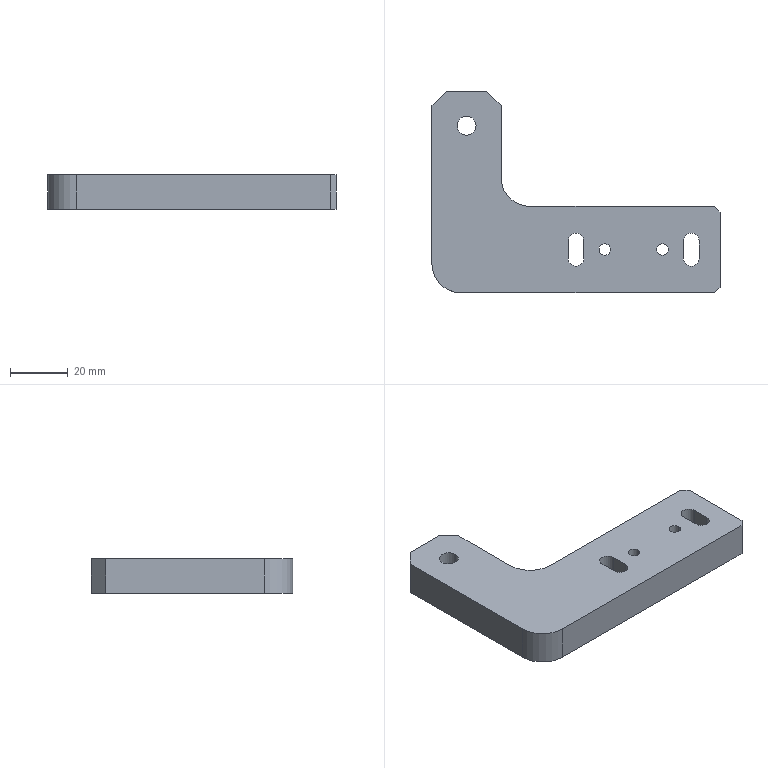Part | STEP file | 2024 Bag feed rotary shaft mounting plate | 1 solid | 31 faces | box 100 x 70 x 12 mm | volume 44684 mm3 | plane 17 | cylinder 14 | commonest cylinder face diameters 4 x4 5.5 x4 6.6 x2 11 x2 20 x2